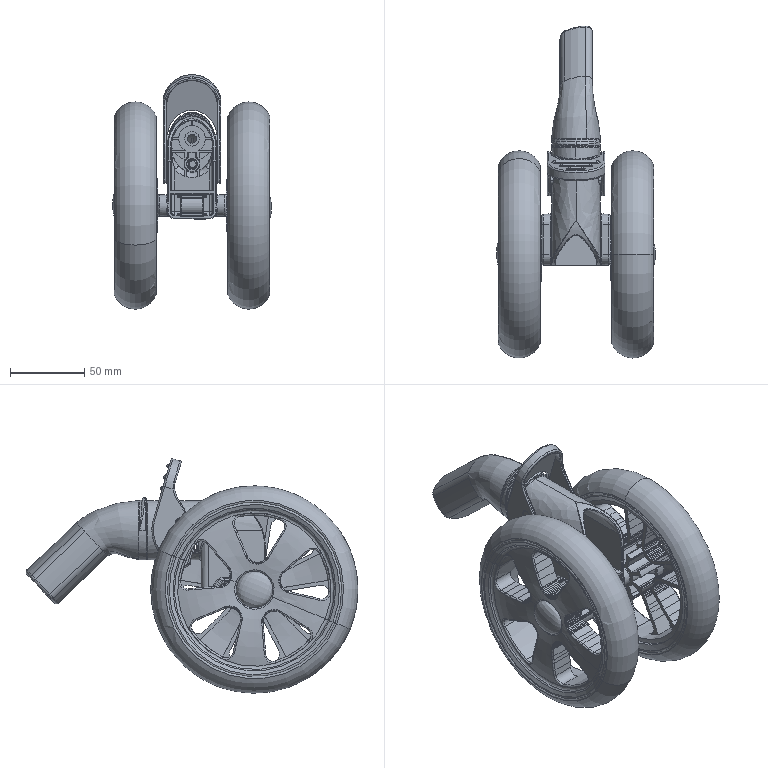Part | SolidWorks | 13 solids | 2365 faces | box 107.069 x 223.806 x 158.072 mm | volume 459720 mm3 | spline 1077 | cylinder 627 | plane 367 | torus 193 | cone 52 | sphere 49 | commonest cylinder face diameters 1 x113 0.6 x108 4 x42 2 x40 10 x35 7 x28